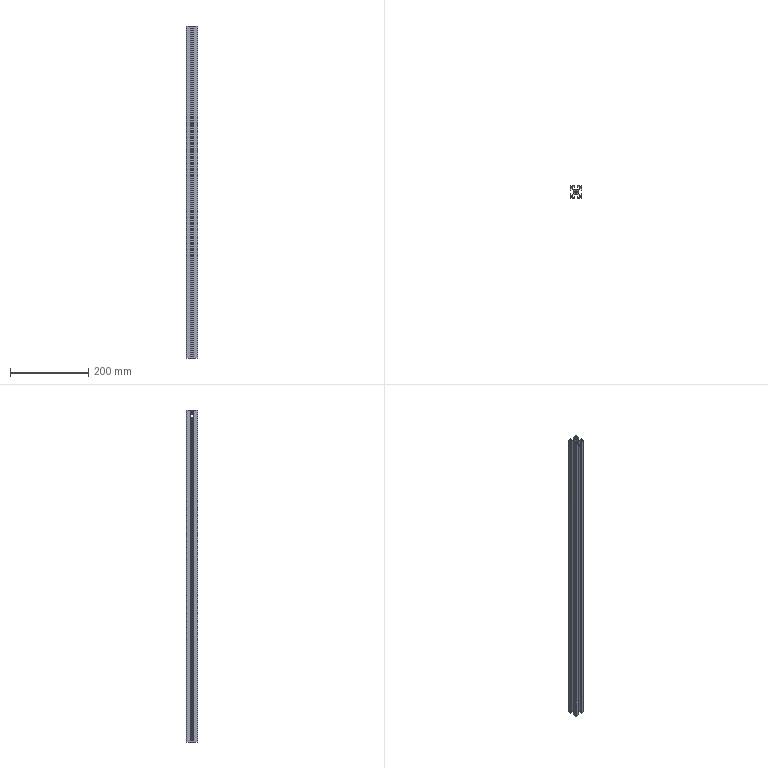Part | STEP file | 227H056139_Default | 1 solid | 106 faces | box 30 x 30 x 850 mm | volume 322963 mm3 | plane 70 | cylinder 36 | commonest cylinder face diameters 0.6 x12 4.2 x8 4 x4 6.8 x4 9 x4 14 x4